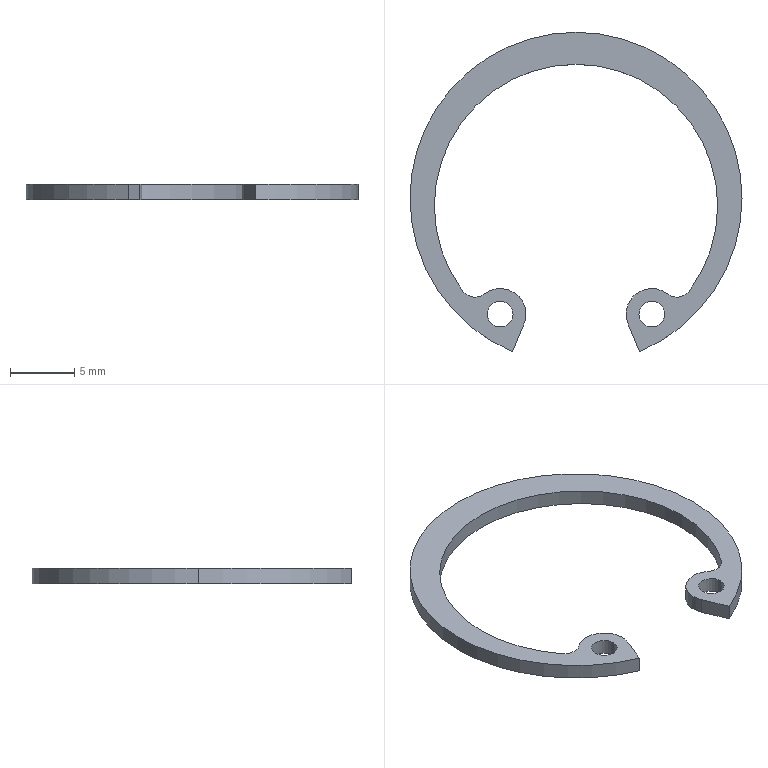Part | STEP file | circlips for holes--type a gb(GB_CONNECTING_PIECE_RING_RRH 24) | 1 solid | 19 faces | box 25.9 x 24.914 x 1.2 mm | volume 171.929 mm3 | cylinder 15 | plane 4 | commonest cylinder face diameters 2 x4 4 x3 22.1 x3 25.9 x3 2.4 x2
STEP:
#1=CARTESIAN_POINT('',(-6.909,-9.04,-1.2));
#2=VERTEX_POINT('',#1);
#3=CARTESIAN_POINT('',(-4.909,-9.04,-1.2));
#4=VERTEX_POINT('',#3);
#5=CARTESIAN_POINT('',(-5.909,-9.04,-1.2));
#6=DIRECTION('',(0.,0.,1.));
#7=DIRECTION('',(1.,0.,0.));
#8=AXIS2_PLACEMENT_3D('',#5,#6,#7);
#9=CIRCLE('',#8,1.);
#10=EDGE_CURVE('',#2,#4,#9,.T.);
#11=ORIENTED_EDGE('',*,*,#10,.F.);
#12=CARTESIAN_POINT('',(-6.909,-9.04,0.));
#13=VERTEX_POINT('',#12);
#14=CARTESIAN_POINT('',(-6.909,-9.04,-1.2));
#15=DIRECTION('',(0.,0.,1.));
#16=VECTOR('',#15,1000.);
#17=LINE('',#14,#16);
#18=EDGE_CURVE('',#2,#13,#17,.T.);
#19=ORIENTED_EDGE('',*,*,#18,.T.);
#20=CARTESIAN_POINT('',(-4.909,-9.04,0.));
#21=VERTEX_POINT('',#20);
#22=CARTESIAN_POINT('',(-5.909,-9.04,0.));
#23=DIRECTION('',(0.,0.,1.));
#24=DIRECTION('',(1.,0.,0.));
#25=AXIS2_PLACEMENT_3D('',#22,#23,#24);
#26=CIRCLE('',#25,1.);
#27=EDGE_CURVE('',#13,#21,#26,.T.);
#28=ORIENTED_EDGE('',*,*,#27,.T.);
#29=CARTESIAN_POINT('',(-4.909,-9.04,-1.2));
#30=DIRECTION('',(0.,0.,1.));
#31=VECTOR('',#30,1000.);
#32=LINE('',#29,#31);
#33=EDGE_CURVE('',#4,#21,#32,.T.);
#34=ORIENTED_EDGE('',*,*,#33,.F.);
#35=EDGE_LOOP('',(#11,#19,#28,#34));
#36=FACE_OUTER_BOUND('',#35,.T.);
#37=CARTESIAN_POINT('',(-5.909,-9.04,-1.2));
#38=DIRECTION('',(0.,0.,1.));
#39=DIRECTION('',(1.,0.,0.));
#40=AXIS2_PLACEMENT_3D('',#37,#38,#39);
#41=CYLINDRICAL_SURFACE('',#40,1.);
#42=ADVANCED_FACE('',(#36),#41,.F.);
#43=CARTESIAN_POINT('',(4.909,-9.04,-1.2));
#44=VERTEX_POINT('',#43);
#45=CARTESIAN_POINT('',(6.909,-9.04,-1.2));
#46=VERTEX_POINT('',#45);
#47=CARTESIAN_POINT('',(5.909,-9.04,-1.2));
#48=DIRECTION('',(0.,0.,1.));
#49=DIRECTION('',(-1.,0.,0.));
#50=AXIS2_PLACEMENT_3D('',#47,#48,#49);
#51=CIRCLE('',#50,1.);
#52=EDGE_CURVE('',#44,#46,#51,.T.);
#53=ORIENTED_EDGE('',*,*,#52,.F.);
#54=CARTESIAN_POINT('',(4.909,-9.04,0.));
#55=VERTEX_POINT('',#54);
#56=CARTESIAN_POINT('',(4.909,-9.04,-1.2));
#57=DIRECTION('',(0.,0.,1.));
#58=VECTOR('',#57,1000.);
#59=LINE('',#56,#58);
#60=EDGE_CURVE('',#44,#55,#59,.T.);
#61=ORIENTED_EDGE('',*,*,#60,.T.);
#62=CARTESIAN_POINT('',(6.909,-9.04,0.));
#63=VERTEX_POINT('',#62);
#64=CARTESIAN_POINT('',(5.909,-9.04,0.));
#65=DIRECTION('',(0.,0.,1.));
#66=DIRECTION('',(-1.,0.,0.));
#67=AXIS2_PLACEMENT_3D('',#64,#65,#66);
#68=CIRCLE('',#67,1.);
#69=EDGE_CURVE('',#55,#63,#68,.T.);
#70=ORIENTED_EDGE('',*,*,#69,.T.);
#71=CARTESIAN_POINT('',(6.909,-9.04,-1.2));
#72=DIRECTION('',(0.,0.,1.));
#73=VECTOR('',#72,1000.);
#74=LINE('',#71,#73);
#75=EDGE_CURVE('',#46,#63,#74,.T.);
#76=ORIENTED_EDGE('',*,*,#75,.F.);
#77=EDGE_LOOP('',(#53,#61,#70,#76));
#78=FACE_OUTER_BOUND('',#77,.T.);
#79=CARTESIAN_POINT('',(5.909,-9.04,-1.2));
#80=DIRECTION('',(0.,0.,1.));
#81=DIRECTION('',(1.,0.,0.));
#82=AXIS2_PLACEMENT_3D('',#79,#80,#81);
#83=CYLINDRICAL_SURFACE('',#82,1.);
#84=ADVANCED_FACE('',(#78),#83,.F.);
#85=CARTESIAN_POINT('',(-4.061,-9.805,-1.2));
#86=VERTEX_POINT('',#85);
#87=CARTESIAN_POINT('',(-3.909,-9.04,-1.2));
#88=VERTEX_POINT('',#87);
#89=CARTESIAN_POINT('',(-5.909,-9.04,-1.2));
#90=DIRECTION('',(0.,0.,1.));
#91=DIRECTION('',(1.,0.,0.));
#92=AXIS2_PLACEMENT_3D('',#89,#90,#91);
#93=CIRCLE('',#92,2.);
#94=EDGE_CURVE('',#86,#88,#93,.T.);
#95=ORIENTED_EDGE('',*,*,#94,.T.);
#96=CARTESIAN_POINT('',(-3.909,-9.04,0.));
#97=VERTEX_POINT('',#96);
#98=CARTESIAN_POINT('',(-3.909,-9.04,-1.2));
#99=DIRECTION('',(0.,0.,1.));
#100=VECTOR('',#99,1000.);
#101=LINE('',#98,#100);
#102=EDGE_CURVE('',#88,#97,#101,.T.);
#103=ORIENTED_EDGE('',*,*,#102,.T.);
#104=CARTESIAN_POINT('',(-4.061,-9.805,0.));
#105=VERTEX_POINT('',#104);
#106=CARTESIAN_POINT('',(-5.909,-9.04,0.));
#107=DIRECTION('',(0.,0.,1.));
#108=DIRECTION('',(1.,0.,0.));
#109=AXIS2_PLACEMENT_3D('',#106,#107,#108);
#110=CIRCLE('',#109,2.);
#111=EDGE_CURVE('',#105,#97,#110,.T.);
#112=ORIENTED_EDGE('',*,*,#111,.F.);
#113=CARTESIAN_POINT('',(-4.061,-9.805,-1.2));
#114=DIRECTION('',(0.,0.,1.));
#115=VECTOR('',#114,1000.);
#116=LINE('',#113,#115);
#117=EDGE_CURVE('',#86,#105,#116,.T.);
#118=ORIENTED_EDGE('',*,*,#117,.F.);
#119=EDGE_LOOP('',(#95,#103,#112,#118));
#120=FACE_OUTER_BOUND('',#119,.T.);
#121=CARTESIAN_POINT('',(-5.909,-9.04,-1.2));
#122=DIRECTION('',(0.,0.,1.));
#123=DIRECTION('',(1.,0.,0.));
#124=AXIS2_PLACEMENT_3D('',#121,#122,#123);
#125=CYLINDRICAL_SURFACE('',#124,2.);
#126=ADVANCED_FACE('',(#120),#125,.T.);
#127=CARTESIAN_POINT('',(-8.835,-7.236,-1.2));
#128=VERTEX_POINT('',#127);
#129=CARTESIAN_POINT('',(-11.05,-0.6,-1.2));
#130=VERTEX_POINT('',#129);
#131=CARTESIAN_POINT('',(0.,-0.6,-1.2));
#132=DIRECTION('',(0.,0.,-1.));
#133=DIRECTION('',(1.,0.,0.));
#134=AXIS2_PLACEMENT_3D('',#131,#132,#133);
#135=CIRCLE('',#134,11.05);
#136=EDGE_CURVE('',#128,#130,#135,.T.);
#137=ORIENTED_EDGE('',*,*,#136,.T.);
#138=CARTESIAN_POINT('',(-11.05,-0.6,0.));
#139=VERTEX_POINT('',#138);
#140=CARTESIAN_POINT('',(-11.05,-0.6,-1.2));
#141=DIRECTION('',(0.,0.,1.));
#142=VECTOR('',#141,1000.);
#143=LINE('',#140,#142);
#144=EDGE_CURVE('',#130,#139,#143,.T.);
#145=ORIENTED_EDGE('',*,*,#144,.T.);
#146=CARTESIAN_POINT('',(-8.835,-7.236,0.));
#147=VERTEX_POINT('',#146);
#148=CARTESIAN_POINT('',(0.,-0.6,0.));
#149=DIRECTION('',(0.,0.,-1.));
#150=DIRECTION('',(1.,0.,0.));
#151=AXIS2_PLACEMENT_3D('',#148,#149,#150);
#152=CIRCLE('',#151,11.05);
#153=EDGE_CURVE('',#147,#139,#152,.T.);
#154=ORIENTED_EDGE('',*,*,#153,.F.);
#155=CARTESIAN_POINT('',(-8.835,-7.236,-1.2));
#156=DIRECTION('',(0.,0.,1.));
#157=VECTOR('',#156,1000.);
#158=LINE('',#155,#157);
#159=EDGE_CURVE('',#128,#147,#158,.T.);
#160=ORIENTED_EDGE('',*,*,#159,.F.);
#161=EDGE_LOOP('',(#137,#145,#154,#160));
#162=FACE_OUTER_BOUND('',#161,.T.);
#163=CARTESIAN_POINT('',(0.,-0.6,-1.2));
#164=DIRECTION('',(0.,0.,1.));
#165=DIRECTION('',(1.,0.,0.));
#166=AXIS2_PLACEMENT_3D('',#163,#164,#165);
#167=CYLINDRICAL_SURFACE('',#166,11.05);
#168=ADVANCED_FACE('',(#162),#167,.F.);
#169=ORIENTED_EDGE('',*,*,#144,.F.);
#170=CARTESIAN_POINT('',(11.05,-0.6,-1.2));
#171=VERTEX_POINT('',#170);
#172=CARTESIAN_POINT('',(0.,-0.6,-1.2));
#173=DIRECTION('',(0.,0.,-1.));
#174=DIRECTION('',(1.,0.,0.));
#175=AXIS2_PLACEMENT_3D('',#172,#173,#174);
#176=CIRCLE('',#175,11.05);
#177=EDGE_CURVE('',#130,#171,#176,.T.);
#178=ORIENTED_EDGE('',*,*,#177,.T.);
#179=CARTESIAN_POINT('',(11.05,-0.6,0.));
#180=VERTEX_POINT('',#179);
#181=CARTESIAN_POINT('',(11.05,-0.6,-1.2));
#182=DIRECTION('',(0.,0.,1.));
#183=VECTOR('',#182,1000.);
#184=LINE('',#181,#183);
#185=EDGE_CURVE('',#171,#180,#184,.T.);
#186=ORIENTED_EDGE('',*,*,#185,.T.);
#187=CARTESIAN_POINT('',(0.,-0.6,0.));
#188=DIRECTION('',(0.,0.,-1.));
#189=DIRECTION('',(1.,0.,0.));
#190=AXIS2_PLACEMENT_3D('',#187,#188,#189);
#191=CIRCLE('',#190,11.05);
#192=EDGE_CURVE('',#139,#180,#191,.T.);
#193=ORIENTED_EDGE('',*,*,#192,.F.);
#194=EDGE_LOOP('',(#169,#178,#186,#193));
#195=FACE_OUTER_BOUND('',#194,.T.);
#196=CARTESIAN_POINT('',(0.,-0.6,-1.2));
#197=DIRECTION('',(0.,0.,1.));
#198=DIRECTION('',(1.,0.,0.));
#199=AXIS2_PLACEMENT_3D('',#196,#197,#198);
#200=CYLINDRICAL_SURFACE('',#199,11.05);
#201=ADVANCED_FACE('',(#195),#200,.F.);
#202=CARTESIAN_POINT('',(12.95,0.,-1.2));
#203=VERTEX_POINT('',#202);
#204=CARTESIAN_POINT('',(-12.95,0.,-1.2));
#205=VERTEX_POINT('',#204);
#206=CARTESIAN_POINT('',(0.,0.,-1.2));
#207=DIRECTION('',(0.,0.,1.));
#208=DIRECTION('',(1.,0.,0.));
#209=AXIS2_PLACEMENT_3D('',#206,#207,#208);
#210=CIRCLE('',#209,12.95);
#211=EDGE_CURVE('',#203,#205,#210,.T.);
#212=ORIENTED_EDGE('',*,*,#211,.T.);
#213=CARTESIAN_POINT('',(-12.95,0.,0.));
#214=VERTEX_POINT('',#213);
#215=CARTESIAN_POINT('',(-12.95,0.,-1.2));
#216=DIRECTION('',(0.,0.,1.));
#217=VECTOR('',#216,1000.);
#218=LINE('',#215,#217);
#219=EDGE_CURVE('',#205,#214,#218,.T.);
#220=ORIENTED_EDGE('',*,*,#219,.T.);
#221=CARTESIAN_POINT('',(12.95,0.,0.));
#222=VERTEX_POINT('',#221);
#223=CARTESIAN_POINT('',(0.,0.,0.));
#224=DIRECTION('',(0.,0.,1.));
#225=DIRECTION('',(1.,0.,0.));
#226=AXIS2_PLACEMENT_3D('',#223,#224,#225);
#227=CIRCLE('',#226,12.95);
#228=EDGE_CURVE('',#222,#214,#227,.T.);
#229=ORIENTED_EDGE('',*,*,#228,.F.);
#230=CARTESIAN_POINT('',(12.95,0.,-1.2));
#231=DIRECTION('',(0.,0.,1.));
#232=VECTOR('',#231,1000.);
#233=LINE('',#230,#232);
#234=EDGE_CURVE('',#203,#222,#233,.T.);
#235=ORIENTED_EDGE('',*,*,#234,.F.);
#236=EDGE_LOOP('',(#212,#220,#229,#235));
#237=FACE_OUTER_BOUND('',#236,.T.);
#238=CARTESIAN_POINT('',(0.,0.,-1.2));
#239=DIRECTION('',(0.,0.,1.));
#240=DIRECTION('',(1.,0.,0.));
#241=AXIS2_PLACEMENT_3D('',#238,#239,#240);
#242=CYLINDRICAL_SURFACE('',#241,12.95);
#243=ADVANCED_FACE('',(#237),#242,.T.);
#244=CARTESIAN_POINT('',(4.956,-11.964,-1.2));
#245=VERTEX_POINT('',#244);
#246=CARTESIAN_POINT('',(0.,0.,-1.2));
#247=DIRECTION('',(0.,0.,1.));
#248=DIRECTION('',(1.,0.,0.));
#249=AXIS2_PLACEMENT_3D('',#246,#247,#248);
#250=CIRCLE('',#249,12.95);
#251=EDGE_CURVE('',#245,#203,#250,.T.);
#252=ORIENTED_EDGE('',*,*,#251,.T.);
#253=ORIENTED_EDGE('',*,*,#234,.T.);
#254=CARTESIAN_POINT('',(4.956,-11.964,0.));
#255=VERTEX_POINT('',#254);
#256=CARTESIAN_POINT('',(0.,0.,0.));
#257=DIRECTION('',(0.,0.,1.));
#258=DIRECTION('',(1.,0.,0.));
#259=AXIS2_PLACEMENT_3D('',#256,#257,#258);
#260=CIRCLE('',#259,12.95);
#261=EDGE_CURVE('',#255,#222,#260,.T.);
#262=ORIENTED_EDGE('',*,*,#261,.F.);
#263=CARTESIAN_POINT('',(4.956,-11.964,-1.2));
#264=DIRECTION('',(0.,0.,1.));
#265=VECTOR('',#264,1000.);
#266=LINE('',#263,#265);
#267=EDGE_CURVE('',#245,#255,#266,.T.);
#268=ORIENTED_EDGE('',*,*,#267,.F.);
#269=EDGE_LOOP('',(#252,#253,#262,#268));
#270=FACE_OUTER_BOUND('',#269,.T.);
#271=CARTESIAN_POINT('',(0.,0.,-1.2));
#272=DIRECTION('',(0.,0.,1.));
#273=DIRECTION('',(1.,0.,0.));
#274=AXIS2_PLACEMENT_3D('',#271,#272,#273);
#275=CYLINDRICAL_SURFACE('',#274,12.95);
#276=ADVANCED_FACE('',(#270),#275,.T.);
#277=ORIENTED_EDGE('',*,*,#219,.F.);
#278=CARTESIAN_POINT('',(-4.956,-11.964,-1.2));
#279=VERTEX_POINT('',#278);
#280=CARTESIAN_POINT('',(0.,0.,-1.2));
#281=DIRECTION('',(0.,0.,1.));
#282=DIRECTION('',(1.,0.,0.));
#283=AXIS2_PLACEMENT_3D('',#280,#281,#282);
#284=CIRCLE('',#283,12.95);
#285=EDGE_CURVE('',#205,#279,#284,.T.);
#286=ORIENTED_EDGE('',*,*,#285,.T.);
#287=CARTESIAN_POINT('',(-4.956,-11.964,0.));
#288=VERTEX_POINT('',#287);
#289=CARTESIAN_POINT('',(-4.956,-11.964,-1.2));
#290=DIRECTION('',(0.,0.,1.));
#291=VECTOR('',#290,1000.);
#292=LINE('',#289,#291);
#293=EDGE_CURVE('',#279,#288,#292,.T.);
#294=ORIENTED_EDGE('',*,*,#293,.T.);
#295=CARTESIAN_POINT('',(0.,0.,0.));
#296=DIRECTION('',(0.,0.,1.));
#297=DIRECTION('',(1.,0.,0.));
#298=AXIS2_PLACEMENT_3D('',#295,#296,#297);
#299=CIRCLE('',#298,12.95);
#300=EDGE_CURVE('',#214,#288,#299,.T.);
#301=ORIENTED_EDGE('',*,*,#300,.F.);
#302=EDGE_LOOP('',(#277,#286,#294,#301));
#303=FACE_OUTER_BOUND('',#302,.T.);
#304=CARTESIAN_POINT('',(0.,0.,-1.2));
#305=DIRECTION('',(0.,0.,1.));
#306=DIRECTION('',(1.,0.,0.));
#307=AXIS2_PLACEMENT_3D('',#304,#305,#306);
#308=CYLINDRICAL_SURFACE('',#307,12.95);
#309=ADVANCED_FACE('',(#303),#308,.T.);
#310=CARTESIAN_POINT('',(4.061,-9.805,0.));
#311=VERTEX_POINT('',#310);
#312=CARTESIAN_POINT('',(4.061,-9.805,0.));
#313=DIRECTION('',(0.3827,-0.9239,0.));
#314=VECTOR('',#313,1000.);
#315=LINE('',#312,#314);
#316=EDGE_CURVE('',#311,#255,#315,.T.);
#317=ORIENTED_EDGE('',*,*,#316,.F.);
#318=CARTESIAN_POINT('',(4.061,-9.805,-1.2));
#319=VERTEX_POINT('',#318);
#320=CARTESIAN_POINT('',(4.061,-9.805,-1.2));
#321=DIRECTION('',(0.,0.,1.));
#322=VECTOR('',#321,1000.);
#323=LINE('',#320,#322);
#324=EDGE_CURVE('',#319,#311,#323,.T.);
#325=ORIENTED_EDGE('',*,*,#324,.F.);
#326=CARTESIAN_POINT('',(4.061,-9.805,-1.2));
#327=DIRECTION('',(0.3827,-0.9239,0.));
#328=VECTOR('',#327,1000.);
#329=LINE('',#326,#328);
#330=EDGE_CURVE('',#319,#245,#329,.T.);
#331=ORIENTED_EDGE('',*,*,#330,.T.);
#332=ORIENTED_EDGE('',*,*,#267,.T.);
#333=EDGE_LOOP('',(#317,#325,#331,#332));
#334=FACE_OUTER_BOUND('',#333,.T.);
#335=CARTESIAN_POINT('',(4.061,-9.805,-1.2));
#336=DIRECTION('',(-0.9239,-0.3827,0.));
#337=DIRECTION('',(0.3827,-0.9239,0.));
#338=AXIS2_PLACEMENT_3D('',#335,#336,#337);
#339=PLANE('',#338);
#340=ADVANCED_FACE('',(#334),#339,.T.);
#341=CARTESIAN_POINT('',(7.138,-7.462,0.));
#342=VERTEX_POINT('',#341);
#343=CARTESIAN_POINT('',(5.909,-9.04,0.));
#344=DIRECTION('',(0.,0.,1.));
#345=DIRECTION('',(-1.,0.,0.));
#346=AXIS2_PLACEMENT_3D('',#343,#344,#345);
#347=CIRCLE('',#346,2.);
#348=EDGE_CURVE('',#342,#311,#347,.T.);
#349=ORIENTED_EDGE('',*,*,#348,.F.);
#350=CARTESIAN_POINT('',(7.138,-7.462,-1.2));
#351=VERTEX_POINT('',#350);
#352=CARTESIAN_POINT('',(7.138,-7.462,-1.2));
#353=DIRECTION('',(0.,0.,1.));
#354=VECTOR('',#353,1000.);
#355=LINE('',#352,#354);
#356=EDGE_CURVE('',#351,#342,#355,.T.);
#357=ORIENTED_EDGE('',*,*,#356,.F.);
#358=CARTESIAN_POINT('',(5.909,-9.04,-1.2));
#359=DIRECTION('',(0.,0.,1.));
#360=DIRECTION('',(-1.,0.,0.));
#361=AXIS2_PLACEMENT_3D('',#358,#359,#360);
#362=CIRCLE('',#361,2.);
#363=EDGE_CURVE('',#351,#319,#362,.T.);
#364=ORIENTED_EDGE('',*,*,#363,.T.);
#365=ORIENTED_EDGE('',*,*,#324,.T.);
#366=EDGE_LOOP('',(#349,#357,#364,#365));
#367=FACE_OUTER_BOUND('',#366,.T.);
#368=CARTESIAN_POINT('',(5.909,-9.04,-1.2));
#369=DIRECTION('',(0.,0.,1.));
#370=DIRECTION('',(1.,0.,0.));
#371=AXIS2_PLACEMENT_3D('',#368,#369,#370);
#372=CYLINDRICAL_SURFACE('',#371,2.);
#373=ADVANCED_FACE('',(#367),#372,.T.);
#374=CARTESIAN_POINT('',(8.835,-7.236,0.));
#375=VERTEX_POINT('',#374);
#376=CARTESIAN_POINT('',(7.876,-6.516,0.));
#377=DIRECTION('',(0.,0.,-1.));
#378=DIRECTION('',(-1.,0.,0.));
#379=AXIS2_PLACEMENT_3D('',#376,#377,#378);
#380=CIRCLE('',#379,1.2);
#381=EDGE_CURVE('',#375,#342,#380,.T.);
#382=ORIENTED_EDGE('',*,*,#381,.F.);
#383=CARTESIAN_POINT('',(8.835,-7.236,-1.2));
#384=VERTEX_POINT('',#383);
#385=CARTESIAN_POINT('',(8.835,-7.236,-1.2));
#386=DIRECTION('',(0.,0.,1.));
#387=VECTOR('',#386,1000.);
#388=LINE('',#385,#387);
#389=EDGE_CURVE('',#384,#375,#388,.T.);
#390=ORIENTED_EDGE('',*,*,#389,.F.);
#391=CARTESIAN_POINT('',(7.876,-6.516,-1.2));
#392=DIRECTION('',(0.,0.,-1.));
#393=DIRECTION('',(-1.,0.,0.));
#394=AXIS2_PLACEMENT_3D('',#391,#392,#393);
#395=CIRCLE('',#394,1.2);
#396=EDGE_CURVE('',#384,#351,#395,.T.);
#397=ORIENTED_EDGE('',*,*,#396,.T.);
#398=ORIENTED_EDGE('',*,*,#356,.T.);
#399=EDGE_LOOP('',(#382,#390,#397,#398));
#400=FACE_OUTER_BOUND('',#399,.T.);
#401=CARTESIAN_POINT('',(7.876,-6.516,-1.2));
#402=DIRECTION('',(0.,0.,1.));
#403=DIRECTION('',(1.,0.,0.));
#404=AXIS2_PLACEMENT_3D('',#401,#402,#403);
#405=CYLINDRICAL_SURFACE('',#404,1.2);
#406=ADVANCED_FACE('',(#400),#405,.F.);
#407=ORIENTED_EDGE('',*,*,#185,.F.);
#408=CARTESIAN_POINT('',(0.,-0.6,-1.2));
#409=DIRECTION('',(0.,0.,-1.));
#410=DIRECTION('',(1.,0.,0.));
#411=AXIS2_PLACEMENT_3D('',#408,#409,#410);
#412=CIRCLE('',#411,11.05);
#413=EDGE_CURVE('',#171,#384,#412,.T.);
#414=ORIENTED_EDGE('',*,*,#413,.T.);
#415=ORIENTED_EDGE('',*,*,#389,.T.);
#416=CARTESIAN_POINT('',(0.,-0.6,0.));
#417=DIRECTION('',(0.,0.,-1.));
#418=DIRECTION('',(1.,0.,0.));
#419=AXIS2_PLACEMENT_3D('',#416,#417,#418);
#420=CIRCLE('',#419,11.05);
#421=EDGE_CURVE('',#180,#375,#420,.T.);
#422=ORIENTED_EDGE('',*,*,#421,.F.);
#423=EDGE_LOOP('',(#407,#414,#415,#422));
#424=FACE_OUTER_BOUND('',#423,.T.);
#425=CARTESIAN_POINT('',(0.,-0.6,-1.2));
#426=DIRECTION('',(0.,0.,1.));
#427=DIRECTION('',(1.,0.,0.));
#428=AXIS2_PLACEMENT_3D('',#425,#426,#427);
#429=CYLINDRICAL_SURFACE('',#428,11.05);
#430=ADVANCED_FACE('',(#424),#429,.F.);
#431=CARTESIAN_POINT('',(-7.138,-7.462,0.));
#432=VERTEX_POINT('',#431);
#433=CARTESIAN_POINT('',(-7.876,-6.516,0.));
#434=DIRECTION('',(0.,0.,-1.));
#435=DIRECTION('',(1.,0.,0.));
#436=AXIS2_PLACEMENT_3D('',#433,#434,#435);
#437=CIRCLE('',#436,1.2);
#438=EDGE_CURVE('',#432,#147,#437,.T.);
#439=ORIENTED_EDGE('',*,*,#438,.F.);
#440=CARTESIAN_POINT('',(-7.138,-7.462,-1.2));
#441=VERTEX_POINT('',#440);
#442=CARTESIAN_POINT('',(-7.138,-7.462,-1.2));
#443=DIRECTION('',(0.,0.,1.));
#444=VECTOR('',#443,1000.);
#445=LINE('',#442,#444);
#446=EDGE_CURVE('',#441,#432,#445,.T.);
#447=ORIENTED_EDGE('',*,*,#446,.F.);
#448=CARTESIAN_POINT('',(-7.876,-6.516,-1.2));
#449=DIRECTION('',(0.,0.,-1.));
#450=DIRECTION('',(1.,0.,0.));
#451=AXIS2_PLACEMENT_3D('',#448,#449,#450);
#452=CIRCLE('',#451,1.2);
#453=EDGE_CURVE('',#441,#128,#452,.T.);
#454=ORIENTED_EDGE('',*,*,#453,.T.);
#455=ORIENTED_EDGE('',*,*,#159,.T.);
#456=EDGE_LOOP('',(#439,#447,#454,#455));
#457=FACE_OUTER_BOUND('',#456,.T.);
#458=CARTESIAN_POINT('',(-7.876,-6.516,-1.2));
#459=DIRECTION('',(0.,0.,1.));
#460=DIRECTION('',(1.,0.,0.));
#461=AXIS2_PLACEMENT_3D('',#458,#459,#460);
#462=CYLINDRICAL_SURFACE('',#461,1.2);
#463=ADVANCED_FACE('',(#457),#462,.F.);
#464=ORIENTED_EDGE('',*,*,#102,.F.);
#465=CARTESIAN_POINT('',(-5.909,-9.04,-1.2));
#466=DIRECTION('',(0.,0.,1.));
#467=DIRECTION('',(1.,0.,0.));
#468=AXIS2_PLACEMENT_3D('',#465,#466,#467);
#469=CIRCLE('',#468,2.);
#470=EDGE_CURVE('',#88,#441,#469,.T.);
#471=ORIENTED_EDGE('',*,*,#470,.T.);
#472=ORIENTED_EDGE('',*,*,#446,.T.);
#473=CARTESIAN_POINT('',(-5.909,-9.04,0.));
#474=DIRECTION('',(0.,0.,1.));
#475=DIRECTION('',(1.,0.,0.));
#476=AXIS2_PLACEMENT_3D('',#473,#474,#475);
#477=CIRCLE('',#476,2.);
#478=EDGE_CURVE('',#97,#432,#477,.T.);
#479=ORIENTED_EDGE('',*,*,#478,.F.);
#480=EDGE_LOOP('',(#464,#471,#472,#479));
#481=FACE_OUTER_BOUND('',#480,.T.);
#482=CARTESIAN_POINT('',(-5.909,-9.04,-1.2));
#483=DIRECTION('',(0.,0.,1.));
#484=DIRECTION('',(1.,0.,0.));
#485=AXIS2_PLACEMENT_3D('',#482,#483,#484);
#486=CYLINDRICAL_SURFACE('',#485,2.);
#487=ADVANCED_FACE('',(#481),#486,.T.);
#488=CARTESIAN_POINT('',(-4.061,-9.805,0.));
#489=DIRECTION('',(0.3827,0.9239,0.));
#490=VECTOR('',#489,1000.);
#491=LINE('',#488,#490);
#492=EDGE_CURVE('',#288,#105,#491,.T.);
#493=ORIENTED_EDGE('',*,*,#492,.F.);
#494=ORIENTED_EDGE('',*,*,#293,.F.);
#495=CARTESIAN_POINT('',(-4.061,-9.805,-1.2));
#496=DIRECTION('',(0.3827,0.9239,0.));
#497=VECTOR('',#496,1000.);
#498=LINE('',#495,#497);
#499=EDGE_CURVE('',#279,#86,#498,.T.);
#500=ORIENTED_EDGE('',*,*,#499,.T.);
#501=ORIENTED_EDGE('',*,*,#117,.T.);
#502=EDGE_LOOP('',(#493,#494,#500,#501));
#503=FACE_OUTER_BOUND('',#502,.T.);
#504=CARTESIAN_POINT('',(-4.061,-9.805,-1.2));
#505=DIRECTION('',(0.9239,-0.3827,0.));
#506=DIRECTION('',(0.3827,0.9239,0.));
#507=AXIS2_PLACEMENT_3D('',#504,#505,#506);
#508=PLANE('',#507);
#509=ADVANCED_FACE('',(#503),#508,.T.);
#510=CARTESIAN_POINT('',(-5.909,-9.04,-1.2));
#511=DIRECTION('',(0.,0.,1.));
#512=DIRECTION('',(1.,0.,0.));
#513=AXIS2_PLACEMENT_3D('',#510,#511,#512);
#514=CIRCLE('',#513,1.);
#515=EDGE_CURVE('',#4,#2,#514,.T.);
#516=ORIENTED_EDGE('',*,*,#515,.T.);
#517=ORIENTED_EDGE('',*,*,#10,.T.);
#518=EDGE_LOOP('',(#516,#517));
#519=FACE_BOUND('',#518,.T.);
#520=CARTESIAN_POINT('',(5.909,-9.04,-1.2));
#521=DIRECTION('',(0.,0.,1.));
#522=DIRECTION('',(-1.,0.,0.));
#523=AXIS2_PLACEMENT_3D('',#520,#521,#522);
#524=CIRCLE('',#523,1.);
#525=EDGE_CURVE('',#46,#44,#524,.T.);
#526=ORIENTED_EDGE('',*,*,#525,.T.);
#527=ORIENTED_EDGE('',*,*,#52,.T.);
#528=EDGE_LOOP('',(#526,#527));
#529=FACE_BOUND('',#528,.T.);
#530=ORIENTED_EDGE('',*,*,#251,.F.);
#531=ORIENTED_EDGE('',*,*,#330,.F.);
#532=ORIENTED_EDGE('',*,*,#363,.F.);
#533=ORIENTED_EDGE('',*,*,#396,.F.);
#534=ORIENTED_EDGE('',*,*,#413,.F.);
#535=ORIENTED_EDGE('',*,*,#177,.F.);
#536=ORIENTED_EDGE('',*,*,#136,.F.);
#537=ORIENTED_EDGE('',*,*,#453,.F.);
#538=ORIENTED_EDGE('',*,*,#470,.F.);
#539=ORIENTED_EDGE('',*,*,#94,.F.);
#540=ORIENTED_EDGE('',*,*,#499,.F.);
#541=ORIENTED_EDGE('',*,*,#285,.F.);
#542=ORIENTED_EDGE('',*,*,#211,.F.);
#543=EDGE_LOOP('',(#530,#531,#532,#533,#534,#535,#536,#537,#538,#539,#540,#541,#542));
#544=FACE_OUTER_BOUND('',#543,.T.);
#545=CARTESIAN_POINT('',(0.,0.,-1.2));
#546=DIRECTION('',(0.,0.,1.));
#547=DIRECTION('',(1.,0.,0.));
#548=AXIS2_PLACEMENT_3D('',#545,#546,#547);
#549=PLANE('',#548);
#550=ADVANCED_FACE('',(#519,#529,#544),#549,.F.);
#551=CARTESIAN_POINT('',(-5.909,-9.04,0.));
#552=DIRECTION('',(0.,0.,1.));
#553=DIRECTION('',(1.,0.,0.));
#554=AXIS2_PLACEMENT_3D('',#551,#552,#553);
#555=CIRCLE('',#554,1.);
#556=EDGE_CURVE('',#21,#13,#555,.T.);
#557=ORIENTED_EDGE('',*,*,#556,.F.);
#558=ORIENTED_EDGE('',*,*,#27,.F.);
#559=EDGE_LOOP('',(#557,#558));
#560=FACE_BOUND('',#559,.T.);
#561=CARTESIAN_POINT('',(5.909,-9.04,0.));
#562=DIRECTION('',(0.,0.,1.));
#563=DIRECTION('',(-1.,0.,0.));
#564=AXIS2_PLACEMENT_3D('',#561,#562,#563);
#565=CIRCLE('',#564,1.);
#566=EDGE_CURVE('',#63,#55,#565,.T.);
#567=ORIENTED_EDGE('',*,*,#566,.F.);
#568=ORIENTED_EDGE('',*,*,#69,.F.);
#569=EDGE_LOOP('',(#567,#568));
#570=FACE_BOUND('',#569,.T.);
#571=ORIENTED_EDGE('',*,*,#261,.T.);
#572=ORIENTED_EDGE('',*,*,#228,.T.);
#573=ORIENTED_EDGE('',*,*,#300,.T.);
#574=ORIENTED_EDGE('',*,*,#492,.T.);
#575=ORIENTED_EDGE('',*,*,#111,.T.);
#576=ORIENTED_EDGE('',*,*,#478,.T.);
#577=ORIENTED_EDGE('',*,*,#438,.T.);
#578=ORIENTED_EDGE('',*,*,#153,.T.);
#579=ORIENTED_EDGE('',*,*,#192,.T.);
#580=ORIENTED_EDGE('',*,*,#421,.T.);
#581=ORIENTED_EDGE('',*,*,#381,.T.);
#582=ORIENTED_EDGE('',*,*,#348,.T.);
#583=ORIENTED_EDGE('',*,*,#316,.T.);
#584=EDGE_LOOP('',(#571,#572,#573,#574,#575,#576,#577,#578,#579,#580,#581,#582,#583));
#585=FACE_OUTER_BOUND('',#584,.T.);
#586=CARTESIAN_POINT('',(0.,0.,0.));
#587=DIRECTION('',(0.,0.,1.));
#588=DIRECTION('',(1.,0.,0.));
#589=AXIS2_PLACEMENT_3D('',#586,#587,#588);
#590=PLANE('',#589);
#591=ADVANCED_FACE('',(#560,#570,#585),#590,.T.);
#592=ORIENTED_EDGE('',*,*,#60,.F.);
#593=ORIENTED_EDGE('',*,*,#525,.F.);
#594=ORIENTED_EDGE('',*,*,#75,.T.);
#595=ORIENTED_EDGE('',*,*,#566,.T.);
#596=EDGE_LOOP('',(#592,#593,#594,#595));
#597=FACE_OUTER_BOUND('',#596,.T.);
#598=CARTESIAN_POINT('',(5.909,-9.04,-1.2));
#599=DIRECTION('',(0.,0.,1.));
#600=DIRECTION('',(1.,0.,0.));
#601=AXIS2_PLACEMENT_3D('',#598,#599,#600);
#602=CYLINDRICAL_SURFACE('',#601,1.);
#603=ADVANCED_FACE('',(#597),#602,.F.);
#604=ORIENTED_EDGE('',*,*,#18,.F.);
#605=ORIENTED_EDGE('',*,*,#515,.F.);
#606=ORIENTED_EDGE('',*,*,#33,.T.);
#607=ORIENTED_EDGE('',*,*,#556,.T.);
#608=EDGE_LOOP('',(#604,#605,#606,#607));
#609=FACE_OUTER_BOUND('',#608,.T.);
#610=CARTESIAN_POINT('',(-5.909,-9.04,-1.2));
#611=DIRECTION('',(0.,0.,1.));
#612=DIRECTION('',(1.,0.,0.));
#613=AXIS2_PLACEMENT_3D('',#610,#611,#612);
#614=CYLINDRICAL_SURFACE('',#613,1.);
#615=ADVANCED_FACE('',(#609),#614,.F.);
#616=CLOSED_SHELL('',(#42,#84,#126,#168,#201,#243,#276,#309,#340,#373,#406,#430,#463,#487,#509,#550,#591,#603,#615));
#617=MANIFOLD_SOLID_BREP('',#616);
#618=CARTESIAN_POINT('',(0.,0.,0.));
#619=DIRECTION('',(0.,0.,1.));
#620=DIRECTION('',(1.,0.,0.));
#621=AXIS2_PLACEMENT_3D('',#618,#619,#620);
#622=(LENGTH_UNIT()NAMED_UNIT(*)SI_UNIT(.MILLI.,.METRE.));
#623=UNCERTAINTY_MEASURE_WITH_UNIT(LENGTH_MEASURE(0.00001),#622,'','');
#624=(NAMED_UNIT(*)PLANE_ANGLE_UNIT()SI_UNIT($,.RADIAN.));
#625=(NAMED_UNIT(*)SI_UNIT($,.STERADIAN.)SOLID_ANGLE_UNIT());
#626=(GEOMETRIC_REPRESENTATION_CONTEXT(3)GLOBAL_UNCERTAINTY_ASSIGNED_CONTEXT((#623))GLOBAL_UNIT_ASSIGNED_CONTEXT((#622,#624,#625))REPRESENTATION_CONTEXT('',''));
#627=ADVANCED_BREP_SHAPE_REPRESENTATION('',(#617,#621),#626);